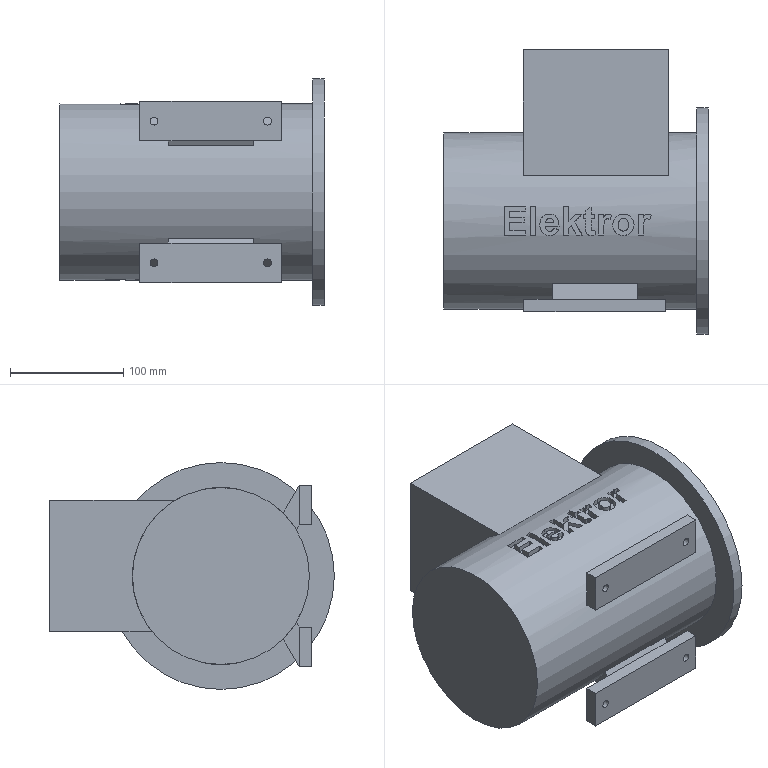Part | STEP file | a-hp_225_37-140_3_0_02 | 1 solid | 238 faces | box 233 x 251 x 200 mm | volume 5912482 mm3 | plane 127 | spline 97 | cylinder 14 | commonest cylinder face diameters 156 x9 7 x4 200 x1